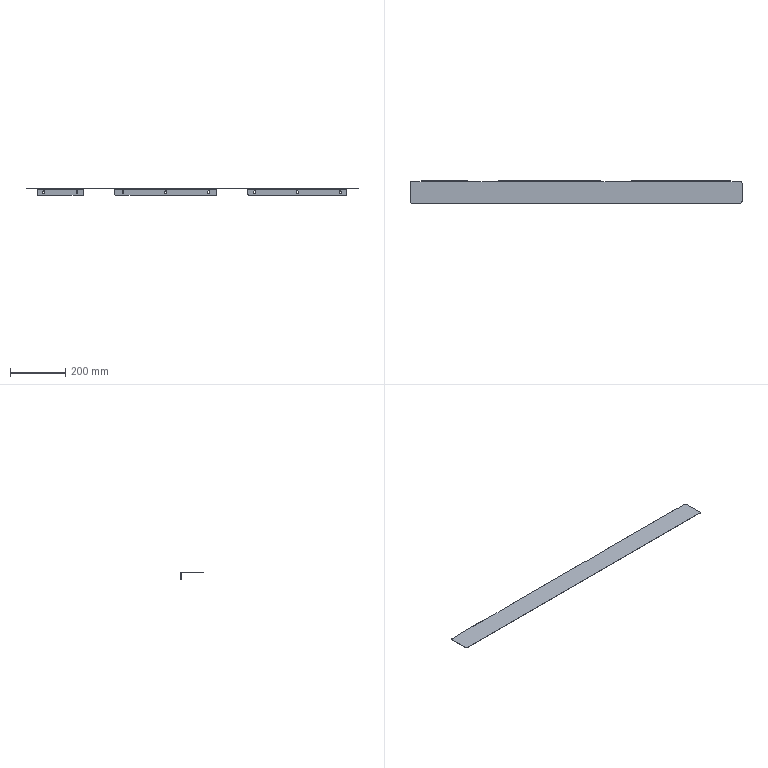Part | SolidWorks | features MoveFace 2, BreakCorner 1, Cut 1, EdgeFlange 1, FlatPattern 1, HoleWzd 1, SMBaseFlange 1, SheetMetal 1 | 1 solid | 92 faces | box 1200 x 80 x 25 mm | volume 115619 mm3 | plane 52 | cylinder 40 | commonest cylinder face diameters 5.8 x24 10 x10 1.473 x3 3.473 x3